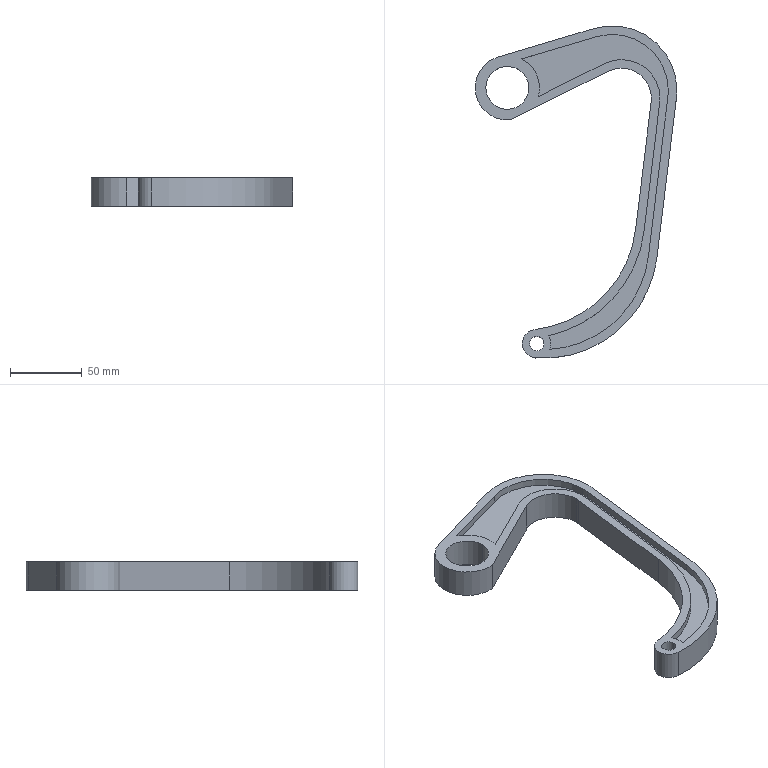Part | SolidWorks | features Extrusion 1, ICE 1 | 1 solid | 48 faces | box 141.009 x 232.349 x 20 mm | volume 138455 mm3 | cylinder 32 | plane 16 | commonest cylinder face diameters 20 x5 45 x5 53.928 x4 78 x4 10 x2 30 x2